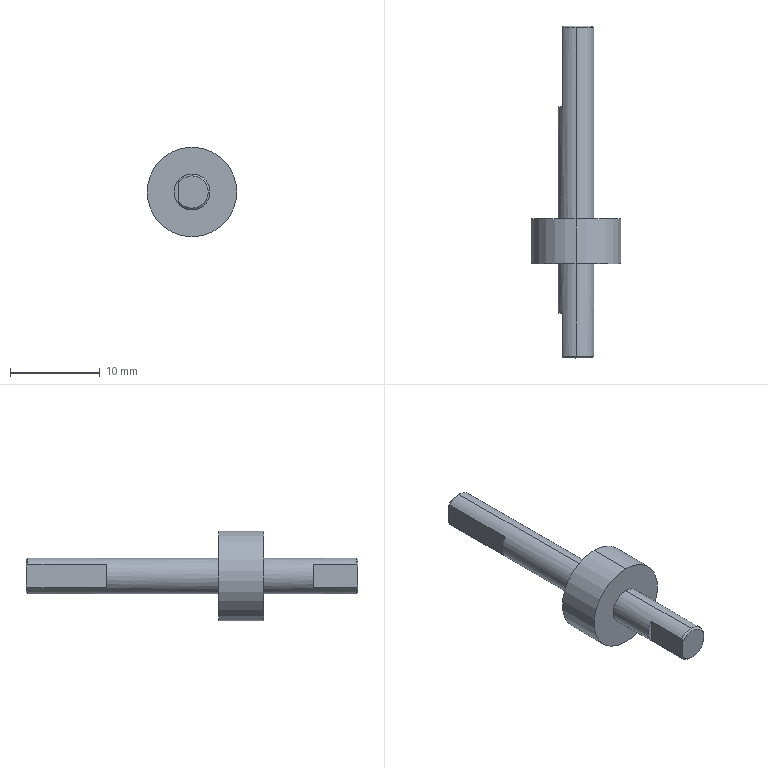Part | NX | 1 solid | 17 faces | box 10 x 37 x 10 mm | volume 781.75 mm3 | plane 8 | cylinder 6 | cone 3 | commonest cylinder face diameters 4 x4 10 x2
STEP:
#1=CARTESIAN_POINT('',(1.8,-13.,0.));
#2=VERTEX_POINT('',#1);
#3=CARTESIAN_POINT('',(2.,-12.8,0.));
#4=VERTEX_POINT('',#3);
#5=CARTESIAN_POINT('',(1.8,-13.,0.));
#6=DIRECTION('',(0.7071,0.7071,0.));
#7=VECTOR('',#6,1000.);
#8=LINE('',#5,#7);
#9=EDGE_CURVE('',#2,#4,#8,.T.);
#10=ORIENTED_EDGE('',*,*,#9,.F.);
#11=CARTESIAN_POINT('',(-1.5,-13.,-0.995));
#12=VERTEX_POINT('',#11);
#13=CARTESIAN_POINT('',(0.,-13.,0.));
#14=DIRECTION('',(0.,-1.,0.));
#15=DIRECTION('',(0.,0.,-1.));
#16=AXIS2_PLACEMENT_3D('',#13,#14,#15);
#17=CIRCLE('',#16,1.8);
#18=EDGE_CURVE('',#12,#2,#17,.T.);
#19=ORIENTED_EDGE('',*,*,#18,.F.);
#20=CARTESIAN_POINT('',(-1.5,-12.8,-1.323));
#21=VERTEX_POINT('',#20);
#22=CARTESIAN_POINT('',(-1.5,-12.8,-1.323));
#23=CARTESIAN_POINT('',(-1.5,-12.818,-1.296));
#24=CARTESIAN_POINT('',(-1.5,-12.835,-1.269));
#25=CARTESIAN_POINT('',(-1.5,-12.852,-1.242));
#26=CARTESIAN_POINT('',(-1.5,-12.869,-1.216));
#27=CARTESIAN_POINT('',(-1.5,-12.886,-1.188));
#28=CARTESIAN_POINT('',(-1.5,-12.903,-1.161));
#29=CARTESIAN_POINT('',(-1.5,-12.92,-1.134));
#30=CARTESIAN_POINT('',(-1.5,-12.936,-1.106));
#31=CARTESIAN_POINT('',(-1.5,-12.952,-1.079));
#32=CARTESIAN_POINT('',(-1.5,-12.969,-1.051));
#33=CARTESIAN_POINT('',(-1.5,-12.984,-1.023));
#34=CARTESIAN_POINT('',(-1.5,-13.,-0.995));
#35=B_SPLINE_CURVE_WITH_KNOTS('',3,(#22,#23,#24,#25,#26,#27,#28,#29,#30,#31,#32,#33,#34),.UNSPECIFIED.,.F.,.F.,(4,3,3,3,4),(0.,0.09586,0.1919,0.288,0.3842),.UNSPECIFIED.);
#36=EDGE_CURVE('',#21,#12,#35,.T.);
#37=ORIENTED_EDGE('',*,*,#36,.F.);
#38=CARTESIAN_POINT('',(0.,-12.8,-2.));
#39=VERTEX_POINT('',#38);
#40=CARTESIAN_POINT('',(0.,-12.8,0.));
#41=DIRECTION('',(0.,1.,0.));
#42=DIRECTION('',(0.,0.,-1.));
#43=AXIS2_PLACEMENT_3D('',#40,#41,#42);
#44=CIRCLE('',#43,2.);
#45=EDGE_CURVE('',#39,#21,#44,.T.);
#46=ORIENTED_EDGE('',*,*,#45,.F.);
#47=CARTESIAN_POINT('',(0.,-12.8,0.));
#48=DIRECTION('',(0.,1.,0.));
#49=DIRECTION('',(0.,0.,-1.));
#50=AXIS2_PLACEMENT_3D('',#47,#48,#49);
#51=CIRCLE('',#50,2.);
#52=EDGE_CURVE('',#4,#39,#51,.T.);
#53=ORIENTED_EDGE('',*,*,#52,.F.);
#54=EDGE_LOOP('',(#10,#19,#37,#46,#53));
#55=FACE_BOUND('',#54,.T.);
#56=CARTESIAN_POINT('',(0.,-13.,0.));
#57=DIRECTION('',(0.,1.,0.));
#58=DIRECTION('',(1.,0.,0.));
#59=AXIS2_PLACEMENT_3D('',#56,#57,#58);
#60=CONICAL_SURFACE('',#59,1.8,0.7854);
#61=ADVANCED_FACE('',(#55),#60,.T.);
#62=CARTESIAN_POINT('',(-1.5,-8.,-1.323));
#63=VERTEX_POINT('',#62);
#64=CARTESIAN_POINT('',(-1.5,0.,-1.323));
#65=DIRECTION('',(0.,-1.,0.));
#66=VECTOR('',#65,1000.);
#67=LINE('',#64,#66);
#68=EDGE_CURVE('',#63,#21,#67,.T.);
#69=ORIENTED_EDGE('',*,*,#68,.T.);
#70=ORIENTED_EDGE('',*,*,#36,.T.);
#71=CARTESIAN_POINT('',(-1.5,-13.,0.995));
#72=VERTEX_POINT('',#71);
#73=CARTESIAN_POINT('',(-1.5,-13.,-5.));
#74=DIRECTION('',(0.,0.,1.));
#75=VECTOR('',#74,1000.);
#76=LINE('',#73,#75);
#77=EDGE_CURVE('',#12,#72,#76,.T.);
#78=ORIENTED_EDGE('',*,*,#77,.T.);
#79=CARTESIAN_POINT('',(-1.5,-12.8,1.323));
#80=VERTEX_POINT('',#79);
#81=CARTESIAN_POINT('',(-1.5,-13.,0.995));
#82=CARTESIAN_POINT('',(-1.5,-12.984,1.023));
#83=CARTESIAN_POINT('',(-1.5,-12.969,1.051));
#84=CARTESIAN_POINT('',(-1.5,-12.953,1.079));
#85=CARTESIAN_POINT('',(-1.5,-12.936,1.106));
#86=CARTESIAN_POINT('',(-1.5,-12.92,1.134));
#87=CARTESIAN_POINT('',(-1.5,-12.903,1.161));
#88=CARTESIAN_POINT('',(-1.5,-12.887,1.188));
#89=CARTESIAN_POINT('',(-1.5,-12.87,1.215));
#90=CARTESIAN_POINT('',(-1.5,-12.852,1.242));
#91=CARTESIAN_POINT('',(-1.5,-12.835,1.269));
#92=CARTESIAN_POINT('',(-1.5,-12.818,1.296));
#93=CARTESIAN_POINT('',(-1.5,-12.8,1.323));
#94=B_SPLINE_CURVE_WITH_KNOTS('',3,(#81,#82,#83,#84,#85,#86,#87,#88,#89,#90,#91,#92,#93),.UNSPECIFIED.,.F.,.F.,(4,3,3,3,4),(0.,0.09611,0.1921,0.2881,0.3842),.UNSPECIFIED.);
#95=EDGE_CURVE('',#72,#80,#94,.T.);
#96=ORIENTED_EDGE('',*,*,#95,.T.);
#97=CARTESIAN_POINT('',(-1.5,-8.,1.323));
#98=VERTEX_POINT('',#97);
#99=CARTESIAN_POINT('',(-1.5,0.,1.323));
#100=DIRECTION('',(0.,1.,0.));
#101=VECTOR('',#100,1000.);
#102=LINE('',#99,#101);
#103=EDGE_CURVE('',#80,#98,#102,.T.);
#104=ORIENTED_EDGE('',*,*,#103,.T.);
#105=CARTESIAN_POINT('',(-1.5,-8.,-5.));
#106=DIRECTION('',(0.,0.,1.));
#107=VECTOR('',#106,1000.);
#108=LINE('',#105,#107);
#109=EDGE_CURVE('',#63,#98,#108,.T.);
#110=ORIENTED_EDGE('',*,*,#109,.F.);
#111=EDGE_LOOP('',(#69,#70,#78,#96,#104,#110));
#112=FACE_BOUND('',#111,.T.);
#113=CARTESIAN_POINT('',(-1.5,-13.,-5.));
#114=DIRECTION('',(1.,0.,0.));
#115=DIRECTION('',(0.,1.,0.));
#116=AXIS2_PLACEMENT_3D('',#113,#114,#115);
#117=PLANE('',#116);
#118=ADVANCED_FACE('',(#112),#117,.F.);
#119=ORIENTED_EDGE('',*,*,#45,.T.);
#120=ORIENTED_EDGE('',*,*,#68,.F.);
#121=CARTESIAN_POINT('',(0.,-8.,0.));
#122=DIRECTION('',(0.,-1.,0.));
#123=DIRECTION('',(0.,0.,1.));
#124=AXIS2_PLACEMENT_3D('',#121,#122,#123);
#125=CIRCLE('',#124,2.);
#126=EDGE_CURVE('',#98,#63,#125,.T.);
#127=ORIENTED_EDGE('',*,*,#126,.F.);
#128=ORIENTED_EDGE('',*,*,#103,.F.);
#129=CARTESIAN_POINT('',(0.,-12.8,2.));
#130=VERTEX_POINT('',#129);
#131=CARTESIAN_POINT('',(0.,-12.8,0.));
#132=DIRECTION('',(0.,1.,0.));
#133=DIRECTION('',(0.,0.,-1.));
#134=AXIS2_PLACEMENT_3D('',#131,#132,#133);
#135=CIRCLE('',#134,2.);
#136=EDGE_CURVE('',#80,#130,#135,.T.);
#137=ORIENTED_EDGE('',*,*,#136,.T.);
#138=CARTESIAN_POINT('',(0.,-2.5,2.));
#139=VERTEX_POINT('',#138);
#140=CARTESIAN_POINT('',(0.,0.,2.));
#141=DIRECTION('',(0.,-1.,0.));
#142=VECTOR('',#141,1000.);
#143=LINE('',#140,#142);
#144=EDGE_CURVE('',#139,#130,#143,.T.);
#145=ORIENTED_EDGE('',*,*,#144,.F.);
#146=CARTESIAN_POINT('',(0.,-2.5,-2.));
#147=VERTEX_POINT('',#146);
#148=CARTESIAN_POINT('',(0.,-2.5,0.));
#149=DIRECTION('',(0.,-1.,0.));
#150=DIRECTION('',(0.,0.,-1.));
#151=AXIS2_PLACEMENT_3D('',#148,#149,#150);
#152=CIRCLE('',#151,2.);
#153=EDGE_CURVE('',#139,#147,#152,.T.);
#154=ORIENTED_EDGE('',*,*,#153,.T.);
#155=CARTESIAN_POINT('',(0.,0.,-2.));
#156=DIRECTION('',(0.,-1.,0.));
#157=VECTOR('',#156,1000.);
#158=LINE('',#155,#157);
#159=EDGE_CURVE('',#147,#39,#158,.T.);
#160=ORIENTED_EDGE('',*,*,#159,.T.);
#161=EDGE_LOOP('',(#119,#120,#127,#128,#137,#145,#154,#160));
#162=FACE_BOUND('',#161,.T.);
#163=CARTESIAN_POINT('',(0.,0.,0.));
#164=DIRECTION('',(0.,-1.,0.));
#165=DIRECTION('',(0.,0.,-1.));
#166=AXIS2_PLACEMENT_3D('',#163,#164,#165);
#167=CYLINDRICAL_SURFACE('',#166,2.);
#168=ADVANCED_FACE('',(#162),#167,.T.);
#169=CARTESIAN_POINT('',(0.,-2.5,5.));
#170=VERTEX_POINT('',#169);
#171=CARTESIAN_POINT('',(0.,-2.5,-5.));
#172=VERTEX_POINT('',#171);
#173=CARTESIAN_POINT('',(0.,-2.5,0.));
#174=DIRECTION('',(0.,-1.,0.));
#175=DIRECTION('',(0.,0.,-1.));
#176=AXIS2_PLACEMENT_3D('',#173,#174,#175);
#177=CIRCLE('',#176,5.);
#178=EDGE_CURVE('',#170,#172,#177,.T.);
#179=ORIENTED_EDGE('',*,*,#178,.F.);
#180=CARTESIAN_POINT('',(0.,2.5,5.));
#181=VERTEX_POINT('',#180);
#182=CARTESIAN_POINT('',(0.,0.,5.));
#183=DIRECTION('',(0.,-1.,0.));
#184=VECTOR('',#183,1000.);
#185=LINE('',#182,#184);
#186=EDGE_CURVE('',#170,#181,#185,.F.);
#187=ORIENTED_EDGE('',*,*,#186,.T.);
#188=CARTESIAN_POINT('',(0.,2.5,-5.));
#189=VERTEX_POINT('',#188);
#190=CARTESIAN_POINT('',(0.,2.5,0.));
#191=DIRECTION('',(0.,-1.,0.));
#192=DIRECTION('',(0.,0.,-1.));
#193=AXIS2_PLACEMENT_3D('',#190,#191,#192);
#194=CIRCLE('',#193,5.);
#195=EDGE_CURVE('',#181,#189,#194,.T.);
#196=ORIENTED_EDGE('',*,*,#195,.T.);
#197=CARTESIAN_POINT('',(0.,0.,-5.));
#198=DIRECTION('',(0.,-1.,0.));
#199=VECTOR('',#198,1000.);
#200=LINE('',#197,#199);
#201=EDGE_CURVE('',#172,#189,#200,.F.);
#202=ORIENTED_EDGE('',*,*,#201,.F.);
#203=EDGE_LOOP('',(#179,#187,#196,#202));
#204=FACE_BOUND('',#203,.T.);
#205=CARTESIAN_POINT('',(0.,0.,0.));
#206=DIRECTION('',(0.,-1.,0.));
#207=DIRECTION('',(0.,0.,-1.));
#208=AXIS2_PLACEMENT_3D('',#205,#206,#207);
#209=CYLINDRICAL_SURFACE('',#208,5.);
#210=ADVANCED_FACE('',(#204),#209,.T.);
#211=CARTESIAN_POINT('',(-1.5,24.,0.995));
#212=VERTEX_POINT('',#211);
#213=CARTESIAN_POINT('',(-1.5,24.,-0.995));
#214=VERTEX_POINT('',#213);
#215=CARTESIAN_POINT('',(0.,24.,0.));
#216=DIRECTION('',(0.,1.,0.));
#217=DIRECTION('',(0.,0.,1.));
#218=AXIS2_PLACEMENT_3D('',#215,#216,#217);
#219=CIRCLE('',#218,1.8);
#220=EDGE_CURVE('',#212,#214,#219,.T.);
#221=ORIENTED_EDGE('',*,*,#220,.F.);
#222=CARTESIAN_POINT('',(-1.5,23.8,1.323));
#223=VERTEX_POINT('',#222);
#224=CARTESIAN_POINT('',(-1.5,24.,0.995));
#225=CARTESIAN_POINT('',(-1.5,23.984,1.023));
#226=CARTESIAN_POINT('',(-1.5,23.969,1.051));
#227=CARTESIAN_POINT('',(-1.5,23.952,1.079));
#228=CARTESIAN_POINT('',(-1.5,23.936,1.106));
#229=CARTESIAN_POINT('',(-1.5,23.92,1.134));
#230=CARTESIAN_POINT('',(-1.5,23.903,1.161));
#231=CARTESIAN_POINT('',(-1.5,23.887,1.188));
#232=CARTESIAN_POINT('',(-1.5,23.87,1.215));
#233=CARTESIAN_POINT('',(-1.5,23.852,1.242));
#234=CARTESIAN_POINT('',(-1.5,23.835,1.269));
#235=CARTESIAN_POINT('',(-1.5,23.818,1.296));
#236=CARTESIAN_POINT('',(-1.5,23.8,1.323));
#237=B_SPLINE_CURVE_WITH_KNOTS('',3,(#224,#225,#226,#227,#228,#229,#230,#231,#232,#233,#234,#235,#236),.UNSPECIFIED.,.F.,.F.,(4,3,3,3,4),(0.,0.09612,0.1921,0.2881,0.3842),.UNSPECIFIED.);
#238=EDGE_CURVE('',#212,#223,#237,.T.);
#239=ORIENTED_EDGE('',*,*,#238,.T.);
#240=CARTESIAN_POINT('',(0.,23.8,2.));
#241=VERTEX_POINT('',#240);
#242=CARTESIAN_POINT('',(0.,23.8,0.));
#243=DIRECTION('',(0.,-1.,0.));
#244=DIRECTION('',(0.,0.,1.));
#245=AXIS2_PLACEMENT_3D('',#242,#243,#244);
#246=CIRCLE('',#245,2.);
#247=EDGE_CURVE('',#241,#223,#246,.T.);
#248=ORIENTED_EDGE('',*,*,#247,.F.);
#249=CARTESIAN_POINT('',(0.,23.8,-2.));
#250=VERTEX_POINT('',#249);
#251=CARTESIAN_POINT('',(0.,23.8,0.));
#252=DIRECTION('',(0.,-1.,0.));
#253=DIRECTION('',(0.,0.,1.));
#254=AXIS2_PLACEMENT_3D('',#251,#252,#253);
#255=CIRCLE('',#254,2.);
#256=EDGE_CURVE('',#250,#241,#255,.T.);
#257=ORIENTED_EDGE('',*,*,#256,.F.);
#258=CARTESIAN_POINT('',(-1.5,23.8,-1.323));
#259=VERTEX_POINT('',#258);
#260=CARTESIAN_POINT('',(0.,23.8,0.));
#261=DIRECTION('',(0.,-1.,0.));
#262=DIRECTION('',(0.,0.,1.));
#263=AXIS2_PLACEMENT_3D('',#260,#261,#262);
#264=CIRCLE('',#263,2.);
#265=EDGE_CURVE('',#259,#250,#264,.T.);
#266=ORIENTED_EDGE('',*,*,#265,.F.);
#267=CARTESIAN_POINT('',(-1.5,23.8,-1.323));
#268=CARTESIAN_POINT('',(-1.5,23.818,-1.296));
#269=CARTESIAN_POINT('',(-1.5,23.835,-1.269));
#270=CARTESIAN_POINT('',(-1.5,23.852,-1.243));
#271=CARTESIAN_POINT('',(-1.5,23.869,-1.216));
#272=CARTESIAN_POINT('',(-1.5,23.886,-1.188));
#273=CARTESIAN_POINT('',(-1.5,23.903,-1.161));
#274=CARTESIAN_POINT('',(-1.5,23.92,-1.134));
#275=CARTESIAN_POINT('',(-1.5,23.936,-1.106));
#276=CARTESIAN_POINT('',(-1.5,23.952,-1.079));
#277=CARTESIAN_POINT('',(-1.5,23.969,-1.051));
#278=CARTESIAN_POINT('',(-1.5,23.984,-1.023));
#279=CARTESIAN_POINT('',(-1.5,24.,-0.995));
#280=B_SPLINE_CURVE_WITH_KNOTS('',3,(#267,#268,#269,#270,#271,#272,#273,#274,#275,#276,#277,#278,#279),.UNSPECIFIED.,.F.,.F.,(4,3,3,3,4),(0.,0.09583,0.1918,0.288,0.3842),.UNSPECIFIED.);
#281=EDGE_CURVE('',#259,#214,#280,.T.);
#282=ORIENTED_EDGE('',*,*,#281,.T.);
#283=EDGE_LOOP('',(#221,#239,#248,#257,#266,#282));
#284=FACE_BOUND('',#283,.T.);
#285=CARTESIAN_POINT('',(0.,23.8,0.));
#286=DIRECTION('',(0.,-1.,0.));
#287=DIRECTION('',(-1.,0.,0.));
#288=AXIS2_PLACEMENT_3D('',#285,#286,#287);
#289=CONICAL_SURFACE('',#288,2.,0.7854);
#290=ADVANCED_FACE('',(#284),#289,.T.);
#291=ORIENTED_EDGE('',*,*,#77,.F.);
#292=ORIENTED_EDGE('',*,*,#18,.T.);
#293=CARTESIAN_POINT('',(0.,-13.,0.));
#294=DIRECTION('',(0.,-1.,0.));
#295=DIRECTION('',(0.,0.,-1.));
#296=AXIS2_PLACEMENT_3D('',#293,#294,#295);
#297=CIRCLE('',#296,1.8);
#298=EDGE_CURVE('',#2,#72,#297,.T.);
#299=ORIENTED_EDGE('',*,*,#298,.T.);
#300=EDGE_LOOP('',(#291,#292,#299));
#301=FACE_BOUND('',#300,.T.);
#302=CARTESIAN_POINT('',(0.,-13.,-2.));
#303=DIRECTION('',(0.,-1.,0.));
#304=DIRECTION('',(0.,0.,-1.));
#305=AXIS2_PLACEMENT_3D('',#302,#303,#304);
#306=PLANE('',#305);
#307=ADVANCED_FACE('',(#301),#306,.T.);
#308=ORIENTED_EDGE('',*,*,#247,.T.);
#309=CARTESIAN_POINT('',(-1.5,15.,1.323));
#310=VERTEX_POINT('',#309);
#311=CARTESIAN_POINT('',(-1.5,0.,1.323));
#312=DIRECTION('',(0.,-1.,0.));
#313=VECTOR('',#312,1000.);
#314=LINE('',#311,#313);
#315=EDGE_CURVE('',#223,#310,#314,.T.);
#316=ORIENTED_EDGE('',*,*,#315,.T.);
#317=CARTESIAN_POINT('',(-1.5,15.,-1.323));
#318=VERTEX_POINT('',#317);
#319=CARTESIAN_POINT('',(0.,15.,0.));
#320=DIRECTION('',(0.,-1.,0.));
#321=DIRECTION('',(0.,0.,1.));
#322=AXIS2_PLACEMENT_3D('',#319,#320,#321);
#323=CIRCLE('',#322,2.);
#324=EDGE_CURVE('',#310,#318,#323,.T.);
#325=ORIENTED_EDGE('',*,*,#324,.T.);
#326=CARTESIAN_POINT('',(-1.5,0.,-1.323));
#327=DIRECTION('',(0.,1.,0.));
#328=VECTOR('',#327,1000.);
#329=LINE('',#326,#328);
#330=EDGE_CURVE('',#318,#259,#329,.T.);
#331=ORIENTED_EDGE('',*,*,#330,.T.);
#332=ORIENTED_EDGE('',*,*,#265,.T.);
#333=CARTESIAN_POINT('',(0.,2.5,-2.));
#334=VERTEX_POINT('',#333);
#335=CARTESIAN_POINT('',(0.,0.,-2.));
#336=DIRECTION('',(0.,-1.,0.));
#337=VECTOR('',#336,1000.);
#338=LINE('',#335,#337);
#339=EDGE_CURVE('',#334,#250,#338,.F.);
#340=ORIENTED_EDGE('',*,*,#339,.F.);
#341=CARTESIAN_POINT('',(0.,2.5,2.));
#342=VERTEX_POINT('',#341);
#343=CARTESIAN_POINT('',(0.,2.5,0.));
#344=DIRECTION('',(0.,-1.,0.));
#345=DIRECTION('',(0.,0.,-1.));
#346=AXIS2_PLACEMENT_3D('',#343,#344,#345);
#347=CIRCLE('',#346,2.);
#348=EDGE_CURVE('',#342,#334,#347,.T.);
#349=ORIENTED_EDGE('',*,*,#348,.F.);
#350=CARTESIAN_POINT('',(0.,0.,2.));
#351=DIRECTION('',(0.,-1.,0.));
#352=VECTOR('',#351,1000.);
#353=LINE('',#350,#352);
#354=EDGE_CURVE('',#342,#241,#353,.F.);
#355=ORIENTED_EDGE('',*,*,#354,.T.);
#356=EDGE_LOOP('',(#308,#316,#325,#331,#332,#340,#349,#355));
#357=FACE_BOUND('',#356,.T.);
#358=CARTESIAN_POINT('',(0.,0.,0.));
#359=DIRECTION('',(0.,-1.,0.));
#360=DIRECTION('',(0.,0.,-1.));
#361=AXIS2_PLACEMENT_3D('',#358,#359,#360);
#362=CYLINDRICAL_SURFACE('',#361,2.);
#363=ADVANCED_FACE('',(#357),#362,.T.);
#364=ORIENTED_EDGE('',*,*,#220,.T.);
#365=CARTESIAN_POINT('',(-1.5,24.,5.));
#366=DIRECTION('',(0.,0.,-1.));
#367=VECTOR('',#366,1000.);
#368=LINE('',#365,#367);
#369=EDGE_CURVE('',#212,#214,#368,.T.);
#370=ORIENTED_EDGE('',*,*,#369,.F.);
#371=EDGE_LOOP('',(#364,#370));
#372=FACE_BOUND('',#371,.T.);
#373=CARTESIAN_POINT('',(0.,24.,0.));
#374=DIRECTION('',(0.,1.,0.));
#375=DIRECTION('',(1.,0.,0.));
#376=AXIS2_PLACEMENT_3D('',#373,#374,#375);
#377=PLANE('',#376);
#378=ADVANCED_FACE('',(#372),#377,.T.);
#379=CARTESIAN_POINT('',(-1.5,15.,5.));
#380=DIRECTION('',(0.,0.,-1.));
#381=VECTOR('',#380,1000.);
#382=LINE('',#379,#381);
#383=EDGE_CURVE('',#310,#318,#382,.T.);
#384=ORIENTED_EDGE('',*,*,#383,.T.);
#385=ORIENTED_EDGE('',*,*,#324,.F.);
#386=EDGE_LOOP('',(#384,#385));
#387=FACE_BOUND('',#386,.T.);
#388=CARTESIAN_POINT('',(-2.,15.,5.));
#389=DIRECTION('',(0.,1.,0.));
#390=DIRECTION('',(1.,0.,0.));
#391=AXIS2_PLACEMENT_3D('',#388,#389,#390);
#392=PLANE('',#391);
#393=ADVANCED_FACE('',(#387),#392,.T.);
#394=ORIENTED_EDGE('',*,*,#383,.F.);
#395=ORIENTED_EDGE('',*,*,#315,.F.);
#396=ORIENTED_EDGE('',*,*,#238,.F.);
#397=ORIENTED_EDGE('',*,*,#369,.T.);
#398=ORIENTED_EDGE('',*,*,#281,.F.);
#399=ORIENTED_EDGE('',*,*,#330,.F.);
#400=EDGE_LOOP('',(#394,#395,#396,#397,#398,#399));
#401=FACE_BOUND('',#400,.T.);
#402=CARTESIAN_POINT('',(-1.5,24.,5.));
#403=DIRECTION('',(-1.,0.,0.));
#404=DIRECTION('',(0.,1.,0.));
#405=AXIS2_PLACEMENT_3D('',#402,#403,#404);
#406=PLANE('',#405);
#407=ADVANCED_FACE('',(#401),#406,.T.);
#408=ORIENTED_EDGE('',*,*,#195,.F.);
#409=CARTESIAN_POINT('',(0.,2.5,0.));
#410=DIRECTION('',(0.,-1.,0.));
#411=DIRECTION('',(0.,0.,-1.));
#412=AXIS2_PLACEMENT_3D('',#409,#410,#411);
#413=CIRCLE('',#412,5.);
#414=EDGE_CURVE('',#189,#181,#413,.T.);
#415=ORIENTED_EDGE('',*,*,#414,.F.);
#416=EDGE_LOOP('',(#408,#415));
#417=FACE_BOUND('',#416,.T.);
#418=ORIENTED_EDGE('',*,*,#348,.T.);
#419=CARTESIAN_POINT('',(0.,2.5,0.));
#420=DIRECTION('',(0.,-1.,0.));
#421=DIRECTION('',(0.,0.,-1.));
#422=AXIS2_PLACEMENT_3D('',#419,#420,#421);
#423=CIRCLE('',#422,2.);
#424=EDGE_CURVE('',#334,#342,#423,.T.);
#425=ORIENTED_EDGE('',*,*,#424,.T.);
#426=EDGE_LOOP('',(#418,#425));
#427=FACE_BOUND('',#426,.T.);
#428=CARTESIAN_POINT('',(0.,2.5,-2.));
#429=DIRECTION('',(0.,1.,0.));
#430=DIRECTION('',(1.,0.,0.));
#431=AXIS2_PLACEMENT_3D('',#428,#429,#430);
#432=PLANE('',#431);
#433=ADVANCED_FACE('',(#417,#427),#432,.T.);
#434=ORIENTED_EDGE('',*,*,#109,.T.);
#435=ORIENTED_EDGE('',*,*,#126,.T.);
#436=EDGE_LOOP('',(#434,#435));
#437=FACE_BOUND('',#436,.T.);
#438=CARTESIAN_POINT('',(-2.,-8.,-5.));
#439=DIRECTION('',(0.,1.,0.));
#440=DIRECTION('',(1.,0.,0.));
#441=AXIS2_PLACEMENT_3D('',#438,#439,#440);
#442=PLANE('',#441);
#443=ADVANCED_FACE('',(#437),#442,.F.);
#444=ORIENTED_EDGE('',*,*,#178,.T.);
#445=CARTESIAN_POINT('',(0.,-2.5,0.));
#446=DIRECTION('',(0.,-1.,0.));
#447=DIRECTION('',(0.,0.,-1.));
#448=AXIS2_PLACEMENT_3D('',#445,#446,#447);
#449=CIRCLE('',#448,5.);
#450=EDGE_CURVE('',#172,#170,#449,.T.);
#451=ORIENTED_EDGE('',*,*,#450,.T.);
#452=EDGE_LOOP('',(#444,#451));
#453=FACE_BOUND('',#452,.T.);
#454=CARTESIAN_POINT('',(0.,-2.5,0.));
#455=DIRECTION('',(0.,-1.,0.));
#456=DIRECTION('',(0.,0.,-1.));
#457=AXIS2_PLACEMENT_3D('',#454,#455,#456);
#458=CIRCLE('',#457,2.);
#459=EDGE_CURVE('',#147,#139,#458,.T.);
#460=ORIENTED_EDGE('',*,*,#459,.F.);
#461=ORIENTED_EDGE('',*,*,#153,.F.);
#462=EDGE_LOOP('',(#460,#461));
#463=FACE_BOUND('',#462,.T.);
#464=CARTESIAN_POINT('',(0.,-2.5,-5.));
#465=DIRECTION('',(0.,-1.,0.));
#466=DIRECTION('',(0.,0.,-1.));
#467=AXIS2_PLACEMENT_3D('',#464,#465,#466);
#468=PLANE('',#467);
#469=ADVANCED_FACE('',(#453,#463),#468,.T.);
#470=ORIENTED_EDGE('',*,*,#339,.T.);
#471=ORIENTED_EDGE('',*,*,#256,.T.);
#472=ORIENTED_EDGE('',*,*,#354,.F.);
#473=ORIENTED_EDGE('',*,*,#424,.F.);
#474=EDGE_LOOP('',(#470,#471,#472,#473));
#475=FACE_BOUND('',#474,.T.);
#476=CARTESIAN_POINT('',(0.,0.,0.));
#477=DIRECTION('',(0.,-1.,0.));
#478=DIRECTION('',(0.,0.,-1.));
#479=AXIS2_PLACEMENT_3D('',#476,#477,#478);
#480=CYLINDRICAL_SURFACE('',#479,2.);
#481=ADVANCED_FACE('',(#475),#480,.T.);
#482=ORIENTED_EDGE('',*,*,#459,.T.);
#483=ORIENTED_EDGE('',*,*,#144,.T.);
#484=CARTESIAN_POINT('',(0.,-12.8,0.));
#485=DIRECTION('',(0.,1.,0.));
#486=DIRECTION('',(0.,0.,-1.));
#487=AXIS2_PLACEMENT_3D('',#484,#485,#486);
#488=CIRCLE('',#487,2.);
#489=EDGE_CURVE('',#130,#4,#488,.T.);
#490=ORIENTED_EDGE('',*,*,#489,.T.);
#491=ORIENTED_EDGE('',*,*,#52,.T.);
#492=ORIENTED_EDGE('',*,*,#159,.F.);
#493=EDGE_LOOP('',(#482,#483,#490,#491,#492));
#494=FACE_BOUND('',#493,.T.);
#495=CARTESIAN_POINT('',(0.,0.,0.));
#496=DIRECTION('',(0.,-1.,0.));
#497=DIRECTION('',(0.,0.,-1.));
#498=AXIS2_PLACEMENT_3D('',#495,#496,#497);
#499=CYLINDRICAL_SURFACE('',#498,2.);
#500=ADVANCED_FACE('',(#494),#499,.T.);
#501=ORIENTED_EDGE('',*,*,#201,.T.);
#502=ORIENTED_EDGE('',*,*,#414,.T.);
#503=ORIENTED_EDGE('',*,*,#186,.F.);
#504=ORIENTED_EDGE('',*,*,#450,.F.);
#505=EDGE_LOOP('',(#501,#502,#503,#504));
#506=FACE_BOUND('',#505,.T.);
#507=CARTESIAN_POINT('',(0.,0.,0.));
#508=DIRECTION('',(0.,-1.,0.));
#509=DIRECTION('',(0.,0.,-1.));
#510=AXIS2_PLACEMENT_3D('',#507,#508,#509);
#511=CYLINDRICAL_SURFACE('',#510,5.);
#512=ADVANCED_FACE('',(#506),#511,.T.);
#513=ORIENTED_EDGE('',*,*,#298,.F.);
#514=ORIENTED_EDGE('',*,*,#9,.T.);
#515=ORIENTED_EDGE('',*,*,#489,.F.);
#516=ORIENTED_EDGE('',*,*,#136,.F.);
#517=ORIENTED_EDGE('',*,*,#95,.F.);
#518=EDGE_LOOP('',(#513,#514,#515,#516,#517));
#519=FACE_BOUND('',#518,.T.);
#520=CARTESIAN_POINT('',(0.,-13.,0.));
#521=DIRECTION('',(0.,1.,0.));
#522=DIRECTION('',(1.,0.,0.));
#523=AXIS2_PLACEMENT_3D('',#520,#521,#522);
#524=CONICAL_SURFACE('',#523,1.8,0.7854);
#525=ADVANCED_FACE('',(#519),#524,.T.);
#526=CLOSED_SHELL('',(#61,#118,#168,#210,#290,#307,#363,#378,#393,#407,#433,#443,#469,#481,#500,#512,#525));
#527=MANIFOLD_SOLID_BREP('',#526);
#528=(LENGTH_UNIT()NAMED_UNIT(*)SI_UNIT(.MILLI.,.METRE.));
#529=UNCERTAINTY_MEASURE_WITH_UNIT(LENGTH_MEASURE(0.00001),#528,'','');
#530=(NAMED_UNIT(*)PLANE_ANGLE_UNIT()SI_UNIT($,.RADIAN.));
#531=(NAMED_UNIT(*)SI_UNIT($,.STERADIAN.)SOLID_ANGLE_UNIT());
#532=(GEOMETRIC_REPRESENTATION_CONTEXT(3)GLOBAL_UNCERTAINTY_ASSIGNED_CONTEXT((#529))GLOBAL_UNIT_ASSIGNED_CONTEXT((#528,#530,#531))REPRESENTATION_CONTEXT('',''));
#533=ADVANCED_BREP_SHAPE_REPRESENTATION('',(#527),#532);